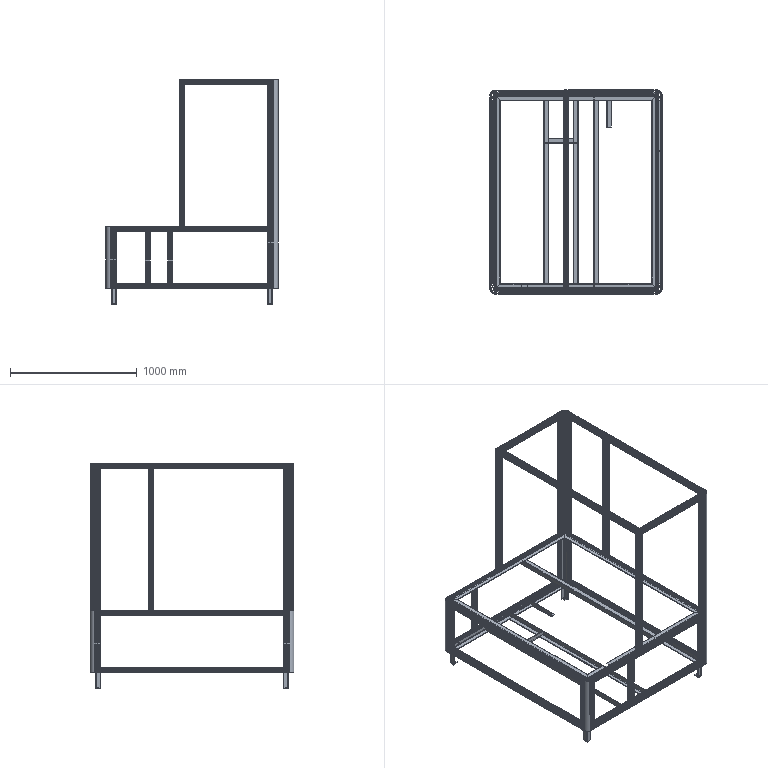Part | 50 solids | 3438 faces | volume 24902953 mm3 | plane 2778 | cylinder 660 | commonest cylinder face diameters 6.8 x176 8.2 x130 5 x112 9 x112 10 x73 3.34 x35